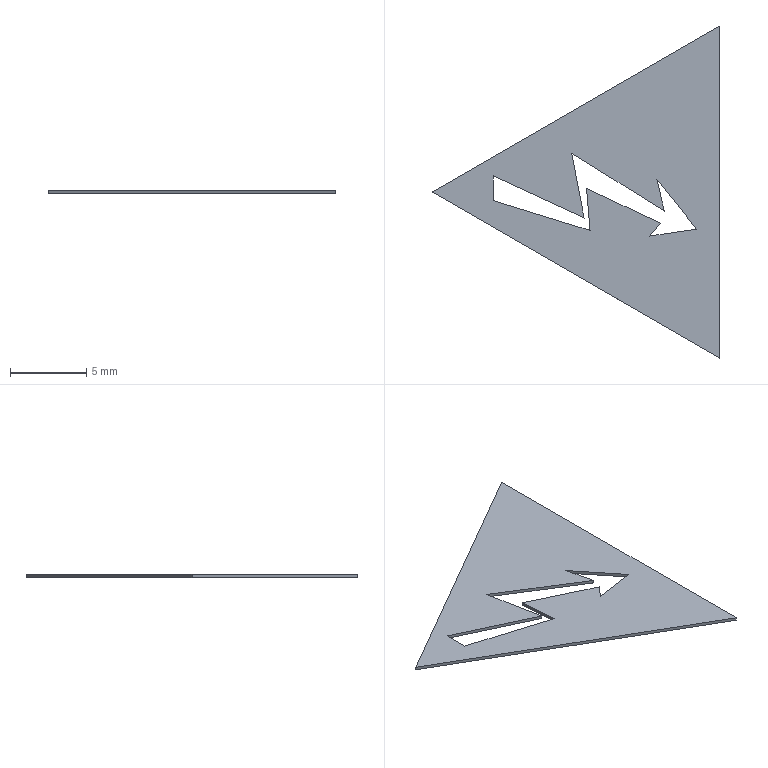Part | SolidWorks | features BaseBody 1 | 1 solid | 16 faces | box 18.841 x 21.756 x 0.2 mm | volume 36.989 mm3 | plane 16
STEP:
#1=CARTESIAN_POINT('',(224.093,-27.499,330.5));
#2=VERTEX_POINT('',#1);
#3=CARTESIAN_POINT('',(221.016,-27.95,330.5));
#4=VERTEX_POINT('',#3);
#5=CARTESIAN_POINT('',(224.093,-27.499,330.5));
#6=DIRECTION('',(-0.9894,-0.145,0.));
#7=VECTOR('',#6,1000.);
#8=LINE('',#5,#7);
#9=EDGE_CURVE('',#2,#4,#8,.T.);
#10=ORIENTED_EDGE('',*,*,#9,.F.);
#11=CARTESIAN_POINT('',(221.487,-24.256,330.5));
#12=VERTEX_POINT('',#11);
#13=CARTESIAN_POINT('',(221.487,-24.256,330.5));
#14=DIRECTION('',(0.6265,-0.7794,0.));
#15=VECTOR('',#14,1000.);
#16=LINE('',#13,#15);
#17=EDGE_CURVE('',#12,#2,#16,.T.);
#18=ORIENTED_EDGE('',*,*,#17,.F.);
#19=CARTESIAN_POINT('',(221.964,-26.319,330.5));
#20=VERTEX_POINT('',#19);
#21=CARTESIAN_POINT('',(221.964,-26.319,330.5));
#22=DIRECTION('',(-0.2253,0.9743,0.));
#23=VECTOR('',#22,1000.);
#24=LINE('',#21,#23);
#25=EDGE_CURVE('',#20,#12,#24,.T.);
#26=ORIENTED_EDGE('',*,*,#25,.F.);
#27=CARTESIAN_POINT('',(215.899,-22.518,330.5));
#28=VERTEX_POINT('',#27);
#29=CARTESIAN_POINT('',(215.899,-22.518,330.5));
#30=DIRECTION('',(0.8473,-0.5311,0.));
#31=VECTOR('',#30,1000.);
#32=LINE('',#29,#31);
#33=EDGE_CURVE('',#28,#20,#32,.T.);
#34=ORIENTED_EDGE('',*,*,#33,.F.);
#35=CARTESIAN_POINT('',(216.713,-26.776,330.5));
#36=VERTEX_POINT('',#35);
#37=CARTESIAN_POINT('',(216.713,-26.776,330.5));
#38=DIRECTION('',(-0.1875,0.9823,0.));
#39=VECTOR('',#38,1000.);
#40=LINE('',#37,#39);
#41=EDGE_CURVE('',#36,#28,#40,.T.);
#42=ORIENTED_EDGE('',*,*,#41,.F.);
#43=CARTESIAN_POINT('',(210.747,-24.01,330.5));
#44=VERTEX_POINT('',#43);
#45=CARTESIAN_POINT('',(210.747,-24.01,330.5));
#46=DIRECTION('',(0.9072,-0.4207,0.));
#47=VECTOR('',#46,1000.);
#48=LINE('',#45,#47);
#49=EDGE_CURVE('',#44,#36,#48,.T.);
#50=ORIENTED_EDGE('',*,*,#49,.F.);
#51=CARTESIAN_POINT('',(210.747,-25.634,330.5));
#52=VERTEX_POINT('',#51);
#53=CARTESIAN_POINT('',(210.747,-25.634,330.5));
#54=DIRECTION('',(0.,1.,0.));
#55=VECTOR('',#54,1000.);
#56=LINE('',#53,#55);
#57=EDGE_CURVE('',#52,#44,#56,.T.);
#58=ORIENTED_EDGE('',*,*,#57,.F.);
#59=CARTESIAN_POINT('',(217.102,-27.586,330.5));
#60=VERTEX_POINT('',#59);
#61=CARTESIAN_POINT('',(217.102,-27.586,330.5));
#62=DIRECTION('',(-0.9559,0.2936,0.));
#63=VECTOR('',#62,1000.);
#64=LINE('',#61,#63);
#65=EDGE_CURVE('',#60,#52,#64,.T.);
#66=ORIENTED_EDGE('',*,*,#65,.F.);
#67=CARTESIAN_POINT('',(216.869,-24.825,330.5));
#68=VERTEX_POINT('',#67);
#69=CARTESIAN_POINT('',(216.869,-24.825,330.5));
#70=DIRECTION('',(0.08386,-0.9965,0.));
#71=VECTOR('',#70,1000.);
#72=LINE('',#69,#71);
#73=EDGE_CURVE('',#68,#60,#72,.T.);
#74=ORIENTED_EDGE('',*,*,#73,.F.);
#75=CARTESIAN_POINT('',(221.715,-27.113,330.5));
#76=VERTEX_POINT('',#75);
#77=CARTESIAN_POINT('',(221.715,-27.113,330.5));
#78=DIRECTION('',(-0.9042,0.4271,0.));
#79=VECTOR('',#78,1000.);
#80=LINE('',#77,#79);
#81=EDGE_CURVE('',#76,#68,#80,.T.);
#82=ORIENTED_EDGE('',*,*,#81,.F.);
#83=CARTESIAN_POINT('',(221.016,-27.95,330.5));
#84=DIRECTION('',(0.6411,0.7674,0.));
#85=VECTOR('',#84,1000.);
#86=LINE('',#83,#85);
#87=EDGE_CURVE('',#4,#76,#86,.T.);
#88=ORIENTED_EDGE('',*,*,#87,.F.);
#89=EDGE_LOOP('',(#10,#18,#26,#34,#42,#50,#58,#66,#74,#82,#88));
#90=FACE_BOUND('',#89,.T.);
#91=CARTESIAN_POINT('',(206.759,-25.066,330.5));
#92=VERTEX_POINT('',#91);
#93=CARTESIAN_POINT('',(225.6,-35.944,330.5));
#94=VERTEX_POINT('',#93);
#95=CARTESIAN_POINT('',(206.759,-25.066,330.5));
#96=DIRECTION('',(0.866,-0.5,0.));
#97=VECTOR('',#96,1000.);
#98=LINE('',#95,#97);
#99=EDGE_CURVE('',#92,#94,#98,.T.);
#100=ORIENTED_EDGE('',*,*,#99,.F.);
#101=CARTESIAN_POINT('',(225.6,-14.188,330.5));
#102=VERTEX_POINT('',#101);
#103=CARTESIAN_POINT('',(225.6,-14.188,330.5));
#104=DIRECTION('',(-0.866,-0.5,0.));
#105=VECTOR('',#104,1000.);
#106=LINE('',#103,#105);
#107=EDGE_CURVE('',#102,#92,#106,.T.);
#108=ORIENTED_EDGE('',*,*,#107,.F.);
#109=CARTESIAN_POINT('',(225.6,-35.944,330.5));
#110=DIRECTION('',(0.,1.,0.));
#111=VECTOR('',#110,1000.);
#112=LINE('',#109,#111);
#113=EDGE_CURVE('',#94,#102,#112,.T.);
#114=ORIENTED_EDGE('',*,*,#113,.F.);
#115=EDGE_LOOP('',(#100,#108,#114));
#116=FACE_OUTER_BOUND('',#115,.T.);
#117=CARTESIAN_POINT('',(253.,-0.0659,330.5));
#118=DIRECTION('',(0.,0.,1.));
#119=DIRECTION('',(1.,0.,0.));
#120=AXIS2_PLACEMENT_3D('',#117,#118,#119);
#121=PLANE('',#120);
#122=ADVANCED_FACE('',(#90,#116),#121,.F.);
#123=CARTESIAN_POINT('',(224.093,-27.499,330.7));
#124=VERTEX_POINT('',#123);
#125=CARTESIAN_POINT('',(221.016,-27.95,330.7));
#126=VERTEX_POINT('',#125);
#127=CARTESIAN_POINT('',(224.093,-27.499,330.7));
#128=DIRECTION('',(-0.9894,-0.145,0.));
#129=VECTOR('',#128,1000.);
#130=LINE('',#127,#129);
#131=EDGE_CURVE('',#124,#126,#130,.T.);
#132=ORIENTED_EDGE('',*,*,#131,.T.);
#133=CARTESIAN_POINT('',(221.715,-27.113,330.7));
#134=VERTEX_POINT('',#133);
#135=CARTESIAN_POINT('',(221.016,-27.95,330.7));
#136=DIRECTION('',(0.6411,0.7674,0.));
#137=VECTOR('',#136,1000.);
#138=LINE('',#135,#137);
#139=EDGE_CURVE('',#126,#134,#138,.T.);
#140=ORIENTED_EDGE('',*,*,#139,.T.);
#141=CARTESIAN_POINT('',(216.869,-24.825,330.7));
#142=VERTEX_POINT('',#141);
#143=CARTESIAN_POINT('',(221.715,-27.113,330.7));
#144=DIRECTION('',(-0.9042,0.4271,0.));
#145=VECTOR('',#144,1000.);
#146=LINE('',#143,#145);
#147=EDGE_CURVE('',#134,#142,#146,.T.);
#148=ORIENTED_EDGE('',*,*,#147,.T.);
#149=CARTESIAN_POINT('',(217.102,-27.586,330.7));
#150=VERTEX_POINT('',#149);
#151=CARTESIAN_POINT('',(216.869,-24.825,330.7));
#152=DIRECTION('',(0.08386,-0.9965,0.));
#153=VECTOR('',#152,1000.);
#154=LINE('',#151,#153);
#155=EDGE_CURVE('',#142,#150,#154,.T.);
#156=ORIENTED_EDGE('',*,*,#155,.T.);
#157=CARTESIAN_POINT('',(210.747,-25.634,330.7));
#158=VERTEX_POINT('',#157);
#159=CARTESIAN_POINT('',(217.102,-27.586,330.7));
#160=DIRECTION('',(-0.9559,0.2936,0.));
#161=VECTOR('',#160,1000.);
#162=LINE('',#159,#161);
#163=EDGE_CURVE('',#150,#158,#162,.T.);
#164=ORIENTED_EDGE('',*,*,#163,.T.);
#165=CARTESIAN_POINT('',(210.747,-24.01,330.7));
#166=VERTEX_POINT('',#165);
#167=CARTESIAN_POINT('',(210.747,-25.634,330.7));
#168=DIRECTION('',(0.,1.,0.));
#169=VECTOR('',#168,1000.);
#170=LINE('',#167,#169);
#171=EDGE_CURVE('',#158,#166,#170,.T.);
#172=ORIENTED_EDGE('',*,*,#171,.T.);
#173=CARTESIAN_POINT('',(216.713,-26.776,330.7));
#174=VERTEX_POINT('',#173);
#175=CARTESIAN_POINT('',(210.747,-24.01,330.7));
#176=DIRECTION('',(0.9072,-0.4207,0.));
#177=VECTOR('',#176,1000.);
#178=LINE('',#175,#177);
#179=EDGE_CURVE('',#166,#174,#178,.T.);
#180=ORIENTED_EDGE('',*,*,#179,.T.);
#181=CARTESIAN_POINT('',(215.899,-22.518,330.7));
#182=VERTEX_POINT('',#181);
#183=CARTESIAN_POINT('',(216.713,-26.776,330.7));
#184=DIRECTION('',(-0.1875,0.9823,0.));
#185=VECTOR('',#184,1000.);
#186=LINE('',#183,#185);
#187=EDGE_CURVE('',#174,#182,#186,.T.);
#188=ORIENTED_EDGE('',*,*,#187,.T.);
#189=CARTESIAN_POINT('',(221.964,-26.319,330.7));
#190=VERTEX_POINT('',#189);
#191=CARTESIAN_POINT('',(215.899,-22.518,330.7));
#192=DIRECTION('',(0.8473,-0.5311,0.));
#193=VECTOR('',#192,1000.);
#194=LINE('',#191,#193);
#195=EDGE_CURVE('',#182,#190,#194,.T.);
#196=ORIENTED_EDGE('',*,*,#195,.T.);
#197=CARTESIAN_POINT('',(221.487,-24.256,330.7));
#198=VERTEX_POINT('',#197);
#199=CARTESIAN_POINT('',(221.964,-26.319,330.7));
#200=DIRECTION('',(-0.2253,0.9743,0.));
#201=VECTOR('',#200,1000.);
#202=LINE('',#199,#201);
#203=EDGE_CURVE('',#190,#198,#202,.T.);
#204=ORIENTED_EDGE('',*,*,#203,.T.);
#205=CARTESIAN_POINT('',(221.487,-24.256,330.7));
#206=DIRECTION('',(0.6265,-0.7794,0.));
#207=VECTOR('',#206,1000.);
#208=LINE('',#205,#207);
#209=EDGE_CURVE('',#198,#124,#208,.T.);
#210=ORIENTED_EDGE('',*,*,#209,.T.);
#211=EDGE_LOOP('',(#132,#140,#148,#156,#164,#172,#180,#188,#196,#204,#210));
#212=FACE_BOUND('',#211,.T.);
#213=CARTESIAN_POINT('',(206.759,-25.066,330.7));
#214=VERTEX_POINT('',#213);
#215=CARTESIAN_POINT('',(225.6,-35.944,330.7));
#216=VERTEX_POINT('',#215);
#217=CARTESIAN_POINT('',(206.759,-25.066,330.7));
#218=DIRECTION('',(0.866,-0.5,0.));
#219=VECTOR('',#218,1000.);
#220=LINE('',#217,#219);
#221=EDGE_CURVE('',#214,#216,#220,.T.);
#222=ORIENTED_EDGE('',*,*,#221,.T.);
#223=CARTESIAN_POINT('',(225.6,-14.188,330.7));
#224=VERTEX_POINT('',#223);
#225=CARTESIAN_POINT('',(225.6,-35.944,330.7));
#226=DIRECTION('',(0.,1.,0.));
#227=VECTOR('',#226,1000.);
#228=LINE('',#225,#227);
#229=EDGE_CURVE('',#216,#224,#228,.T.);
#230=ORIENTED_EDGE('',*,*,#229,.T.);
#231=CARTESIAN_POINT('',(225.6,-14.188,330.7));
#232=DIRECTION('',(-0.866,-0.5,0.));
#233=VECTOR('',#232,1000.);
#234=LINE('',#231,#233);
#235=EDGE_CURVE('',#224,#214,#234,.T.);
#236=ORIENTED_EDGE('',*,*,#235,.T.);
#237=EDGE_LOOP('',(#222,#230,#236));
#238=FACE_OUTER_BOUND('',#237,.T.);
#239=CARTESIAN_POINT('',(253.,-0.0659,330.7));
#240=DIRECTION('',(0.,0.,1.));
#241=DIRECTION('',(1.,0.,0.));
#242=AXIS2_PLACEMENT_3D('',#239,#240,#241);
#243=PLANE('',#242);
#244=ADVANCED_FACE('',(#212,#238),#243,.T.);
#245=ORIENTED_EDGE('',*,*,#17,.T.);
#246=CARTESIAN_POINT('',(224.093,-27.499,330.7));
#247=DIRECTION('',(0.,0.,-1.));
#248=VECTOR('',#247,1000.);
#249=LINE('',#246,#248);
#250=EDGE_CURVE('',#124,#2,#249,.T.);
#251=ORIENTED_EDGE('',*,*,#250,.F.);
#252=ORIENTED_EDGE('',*,*,#209,.F.);
#253=CARTESIAN_POINT('',(221.487,-24.256,330.7));
#254=DIRECTION('',(0.,0.,-1.));
#255=VECTOR('',#254,1000.);
#256=LINE('',#253,#255);
#257=EDGE_CURVE('',#198,#12,#256,.T.);
#258=ORIENTED_EDGE('',*,*,#257,.T.);
#259=EDGE_LOOP('',(#245,#251,#252,#258));
#260=FACE_OUTER_BOUND('',#259,.T.);
#261=CARTESIAN_POINT('',(221.487,-24.256,330.7));
#262=DIRECTION('',(0.7794,0.6265,0.));
#263=DIRECTION('',(0.,0.,-1.));
#264=AXIS2_PLACEMENT_3D('',#261,#262,#263);
#265=PLANE('',#264);
#266=ADVANCED_FACE('',(#260),#265,.F.);
#267=ORIENTED_EDGE('',*,*,#107,.T.);
#268=CARTESIAN_POINT('',(206.759,-25.066,330.7));
#269=DIRECTION('',(0.,0.,-1.));
#270=VECTOR('',#269,1000.);
#271=LINE('',#268,#270);
#272=EDGE_CURVE('',#214,#92,#271,.T.);
#273=ORIENTED_EDGE('',*,*,#272,.F.);
#274=ORIENTED_EDGE('',*,*,#235,.F.);
#275=CARTESIAN_POINT('',(225.6,-14.188,330.7));
#276=DIRECTION('',(0.,0.,-1.));
#277=VECTOR('',#276,1000.);
#278=LINE('',#275,#277);
#279=EDGE_CURVE('',#224,#102,#278,.T.);
#280=ORIENTED_EDGE('',*,*,#279,.T.);
#281=EDGE_LOOP('',(#267,#273,#274,#280));
#282=FACE_OUTER_BOUND('',#281,.T.);
#283=CARTESIAN_POINT('',(225.6,-14.188,330.7));
#284=DIRECTION('',(0.5,-0.866,0.));
#285=DIRECTION('',(0.,0.,-1.));
#286=AXIS2_PLACEMENT_3D('',#283,#284,#285);
#287=PLANE('',#286);
#288=ADVANCED_FACE('',(#282),#287,.F.);
#289=ORIENTED_EDGE('',*,*,#113,.T.);
#290=ORIENTED_EDGE('',*,*,#279,.F.);
#291=ORIENTED_EDGE('',*,*,#229,.F.);
#292=CARTESIAN_POINT('',(225.6,-35.944,330.7));
#293=DIRECTION('',(0.,0.,-1.));
#294=VECTOR('',#293,1000.);
#295=LINE('',#292,#294);
#296=EDGE_CURVE('',#216,#94,#295,.T.);
#297=ORIENTED_EDGE('',*,*,#296,.T.);
#298=EDGE_LOOP('',(#289,#290,#291,#297));
#299=FACE_OUTER_BOUND('',#298,.T.);
#300=CARTESIAN_POINT('',(225.6,-35.944,330.7));
#301=DIRECTION('',(-1.,0.,0.));
#302=DIRECTION('',(0.,0.,1.));
#303=AXIS2_PLACEMENT_3D('',#300,#301,#302);
#304=PLANE('',#303);
#305=ADVANCED_FACE('',(#299),#304,.F.);
#306=ORIENTED_EDGE('',*,*,#99,.T.);
#307=ORIENTED_EDGE('',*,*,#296,.F.);
#308=ORIENTED_EDGE('',*,*,#221,.F.);
#309=ORIENTED_EDGE('',*,*,#272,.T.);
#310=EDGE_LOOP('',(#306,#307,#308,#309));
#311=FACE_OUTER_BOUND('',#310,.T.);
#312=CARTESIAN_POINT('',(206.759,-25.066,330.7));
#313=DIRECTION('',(0.5,0.866,0.));
#314=DIRECTION('',(0.,0.,-1.));
#315=AXIS2_PLACEMENT_3D('',#312,#313,#314);
#316=PLANE('',#315);
#317=ADVANCED_FACE('',(#311),#316,.F.);
#318=ORIENTED_EDGE('',*,*,#25,.T.);
#319=ORIENTED_EDGE('',*,*,#257,.F.);
#320=ORIENTED_EDGE('',*,*,#203,.F.);
#321=CARTESIAN_POINT('',(221.964,-26.319,330.7));
#322=DIRECTION('',(0.,0.,-1.));
#323=VECTOR('',#322,1000.);
#324=LINE('',#321,#323);
#325=EDGE_CURVE('',#190,#20,#324,.T.);
#326=ORIENTED_EDGE('',*,*,#325,.T.);
#327=EDGE_LOOP('',(#318,#319,#320,#326));
#328=FACE_OUTER_BOUND('',#327,.T.);
#329=CARTESIAN_POINT('',(221.964,-26.319,330.7));
#330=DIRECTION('',(-0.9743,-0.2253,0.));
#331=DIRECTION('',(-0.2253,0.9743,0.));
#332=AXIS2_PLACEMENT_3D('',#329,#330,#331);
#333=PLANE('',#332);
#334=ADVANCED_FACE('',(#328),#333,.F.);
#335=ORIENTED_EDGE('',*,*,#33,.T.);
#336=ORIENTED_EDGE('',*,*,#325,.F.);
#337=ORIENTED_EDGE('',*,*,#195,.F.);
#338=CARTESIAN_POINT('',(215.899,-22.518,330.7));
#339=DIRECTION('',(0.,0.,-1.));
#340=VECTOR('',#339,1000.);
#341=LINE('',#338,#340);
#342=EDGE_CURVE('',#182,#28,#341,.T.);
#343=ORIENTED_EDGE('',*,*,#342,.T.);
#344=EDGE_LOOP('',(#335,#336,#337,#343));
#345=FACE_OUTER_BOUND('',#344,.T.);
#346=CARTESIAN_POINT('',(215.899,-22.518,330.7));
#347=DIRECTION('',(0.5311,0.8473,0.));
#348=DIRECTION('',(0.,0.,-1.));
#349=AXIS2_PLACEMENT_3D('',#346,#347,#348);
#350=PLANE('',#349);
#351=ADVANCED_FACE('',(#345),#350,.F.);
#352=ORIENTED_EDGE('',*,*,#41,.T.);
#353=ORIENTED_EDGE('',*,*,#342,.F.);
#354=ORIENTED_EDGE('',*,*,#187,.F.);
#355=CARTESIAN_POINT('',(216.713,-26.776,330.7));
#356=DIRECTION('',(0.,0.,-1.));
#357=VECTOR('',#356,1000.);
#358=LINE('',#355,#357);
#359=EDGE_CURVE('',#174,#36,#358,.T.);
#360=ORIENTED_EDGE('',*,*,#359,.T.);
#361=EDGE_LOOP('',(#352,#353,#354,#360));
#362=FACE_OUTER_BOUND('',#361,.T.);
#363=CARTESIAN_POINT('',(216.713,-26.776,330.7));
#364=DIRECTION('',(-0.9823,-0.1875,0.));
#365=DIRECTION('',(-0.1875,0.9823,0.));
#366=AXIS2_PLACEMENT_3D('',#363,#364,#365);
#367=PLANE('',#366);
#368=ADVANCED_FACE('',(#362),#367,.F.);
#369=ORIENTED_EDGE('',*,*,#49,.T.);
#370=ORIENTED_EDGE('',*,*,#359,.F.);
#371=ORIENTED_EDGE('',*,*,#179,.F.);
#372=CARTESIAN_POINT('',(210.747,-24.01,330.7));
#373=DIRECTION('',(0.,0.,-1.));
#374=VECTOR('',#373,1000.);
#375=LINE('',#372,#374);
#376=EDGE_CURVE('',#166,#44,#375,.T.);
#377=ORIENTED_EDGE('',*,*,#376,.T.);
#378=EDGE_LOOP('',(#369,#370,#371,#377));
#379=FACE_OUTER_BOUND('',#378,.T.);
#380=CARTESIAN_POINT('',(210.747,-24.01,330.7));
#381=DIRECTION('',(0.4207,0.9072,0.));
#382=DIRECTION('',(0.,0.,-1.));
#383=AXIS2_PLACEMENT_3D('',#380,#381,#382);
#384=PLANE('',#383);
#385=ADVANCED_FACE('',(#379),#384,.F.);
#386=ORIENTED_EDGE('',*,*,#57,.T.);
#387=ORIENTED_EDGE('',*,*,#376,.F.);
#388=ORIENTED_EDGE('',*,*,#171,.F.);
#389=CARTESIAN_POINT('',(210.747,-25.634,330.7));
#390=DIRECTION('',(0.,0.,-1.));
#391=VECTOR('',#390,1000.);
#392=LINE('',#389,#391);
#393=EDGE_CURVE('',#158,#52,#392,.T.);
#394=ORIENTED_EDGE('',*,*,#393,.T.);
#395=EDGE_LOOP('',(#386,#387,#388,#394));
#396=FACE_OUTER_BOUND('',#395,.T.);
#397=CARTESIAN_POINT('',(210.747,-25.634,330.7));
#398=DIRECTION('',(-1.,0.,0.));
#399=DIRECTION('',(0.,0.,1.));
#400=AXIS2_PLACEMENT_3D('',#397,#398,#399);
#401=PLANE('',#400);
#402=ADVANCED_FACE('',(#396),#401,.F.);
#403=ORIENTED_EDGE('',*,*,#65,.T.);
#404=ORIENTED_EDGE('',*,*,#393,.F.);
#405=ORIENTED_EDGE('',*,*,#163,.F.);
#406=CARTESIAN_POINT('',(217.102,-27.586,330.7));
#407=DIRECTION('',(0.,0.,-1.));
#408=VECTOR('',#407,1000.);
#409=LINE('',#406,#408);
#410=EDGE_CURVE('',#150,#60,#409,.T.);
#411=ORIENTED_EDGE('',*,*,#410,.T.);
#412=EDGE_LOOP('',(#403,#404,#405,#411));
#413=FACE_OUTER_BOUND('',#412,.T.);
#414=CARTESIAN_POINT('',(217.102,-27.586,330.7));
#415=DIRECTION('',(-0.2936,-0.9559,0.));
#416=DIRECTION('',(-0.9559,0.2936,0.));
#417=AXIS2_PLACEMENT_3D('',#414,#415,#416);
#418=PLANE('',#417);
#419=ADVANCED_FACE('',(#413),#418,.F.);
#420=ORIENTED_EDGE('',*,*,#73,.T.);
#421=ORIENTED_EDGE('',*,*,#410,.F.);
#422=ORIENTED_EDGE('',*,*,#155,.F.);
#423=CARTESIAN_POINT('',(216.869,-24.825,330.7));
#424=DIRECTION('',(0.,0.,-1.));
#425=VECTOR('',#424,1000.);
#426=LINE('',#423,#425);
#427=EDGE_CURVE('',#142,#68,#426,.T.);
#428=ORIENTED_EDGE('',*,*,#427,.T.);
#429=EDGE_LOOP('',(#420,#421,#422,#428));
#430=FACE_OUTER_BOUND('',#429,.T.);
#431=CARTESIAN_POINT('',(216.869,-24.825,330.7));
#432=DIRECTION('',(0.9965,0.08386,0.));
#433=DIRECTION('',(0.,0.,-1.));
#434=AXIS2_PLACEMENT_3D('',#431,#432,#433);
#435=PLANE('',#434);
#436=ADVANCED_FACE('',(#430),#435,.F.);
#437=ORIENTED_EDGE('',*,*,#81,.T.);
#438=ORIENTED_EDGE('',*,*,#427,.F.);
#439=ORIENTED_EDGE('',*,*,#147,.F.);
#440=CARTESIAN_POINT('',(221.715,-27.113,330.7));
#441=DIRECTION('',(0.,0.,-1.));
#442=VECTOR('',#441,1000.);
#443=LINE('',#440,#442);
#444=EDGE_CURVE('',#134,#76,#443,.T.);
#445=ORIENTED_EDGE('',*,*,#444,.T.);
#446=EDGE_LOOP('',(#437,#438,#439,#445));
#447=FACE_OUTER_BOUND('',#446,.T.);
#448=CARTESIAN_POINT('',(221.715,-27.113,330.7));
#449=DIRECTION('',(-0.4271,-0.9042,0.));
#450=DIRECTION('',(-0.9042,0.4271,0.));
#451=AXIS2_PLACEMENT_3D('',#448,#449,#450);
#452=PLANE('',#451);
#453=ADVANCED_FACE('',(#447),#452,.F.);
#454=ORIENTED_EDGE('',*,*,#87,.T.);
#455=ORIENTED_EDGE('',*,*,#444,.F.);
#456=ORIENTED_EDGE('',*,*,#139,.F.);
#457=CARTESIAN_POINT('',(221.016,-27.95,330.7));
#458=DIRECTION('',(0.,0.,-1.));
#459=VECTOR('',#458,1000.);
#460=LINE('',#457,#459);
#461=EDGE_CURVE('',#126,#4,#460,.T.);
#462=ORIENTED_EDGE('',*,*,#461,.T.);
#463=EDGE_LOOP('',(#454,#455,#456,#462));
#464=FACE_OUTER_BOUND('',#463,.T.);
#465=CARTESIAN_POINT('',(221.016,-27.95,330.7));
#466=DIRECTION('',(-0.7674,0.6411,0.));
#467=DIRECTION('',(0.,0.,1.));
#468=AXIS2_PLACEMENT_3D('',#465,#466,#467);
#469=PLANE('',#468);
#470=ADVANCED_FACE('',(#464),#469,.F.);
#471=ORIENTED_EDGE('',*,*,#9,.T.);
#472=ORIENTED_EDGE('',*,*,#461,.F.);
#473=ORIENTED_EDGE('',*,*,#131,.F.);
#474=ORIENTED_EDGE('',*,*,#250,.T.);
#475=EDGE_LOOP('',(#471,#472,#473,#474));
#476=FACE_OUTER_BOUND('',#475,.T.);
#477=CARTESIAN_POINT('',(224.093,-27.499,330.7));
#478=DIRECTION('',(0.145,-0.9894,0.));
#479=DIRECTION('',(0.,0.,-1.));
#480=AXIS2_PLACEMENT_3D('',#477,#478,#479);
#481=PLANE('',#480);
#482=ADVANCED_FACE('',(#476),#481,.F.);
#483=CLOSED_SHELL('',(#122,#244,#266,#288,#305,#317,#334,#351,#368,#385,#402,#419,#436,#453,#470,#482));
#484=MANIFOLD_SOLID_BREP('',#483);
#485=CARTESIAN_POINT('',(0.,0.,0.));
#486=DIRECTION('',(0.,0.,1.));
#487=DIRECTION('',(1.,0.,0.));
#488=AXIS2_PLACEMENT_3D('',#485,#486,#487);
#489=(LENGTH_UNIT()NAMED_UNIT(*)SI_UNIT(.MILLI.,.METRE.));
#490=UNCERTAINTY_MEASURE_WITH_UNIT(LENGTH_MEASURE(0.00001),#489,'','');
#491=(NAMED_UNIT(*)PLANE_ANGLE_UNIT()SI_UNIT($,.RADIAN.));
#492=(NAMED_UNIT(*)SI_UNIT($,.STERADIAN.)SOLID_ANGLE_UNIT());
#493=(GEOMETRIC_REPRESENTATION_CONTEXT(3)GLOBAL_UNCERTAINTY_ASSIGNED_CONTEXT((#490))GLOBAL_UNIT_ASSIGNED_CONTEXT((#489,#491,#492))REPRESENTATION_CONTEXT('',''));
#494=ADVANCED_BREP_SHAPE_REPRESENTATION('',(#484,#488),#493);